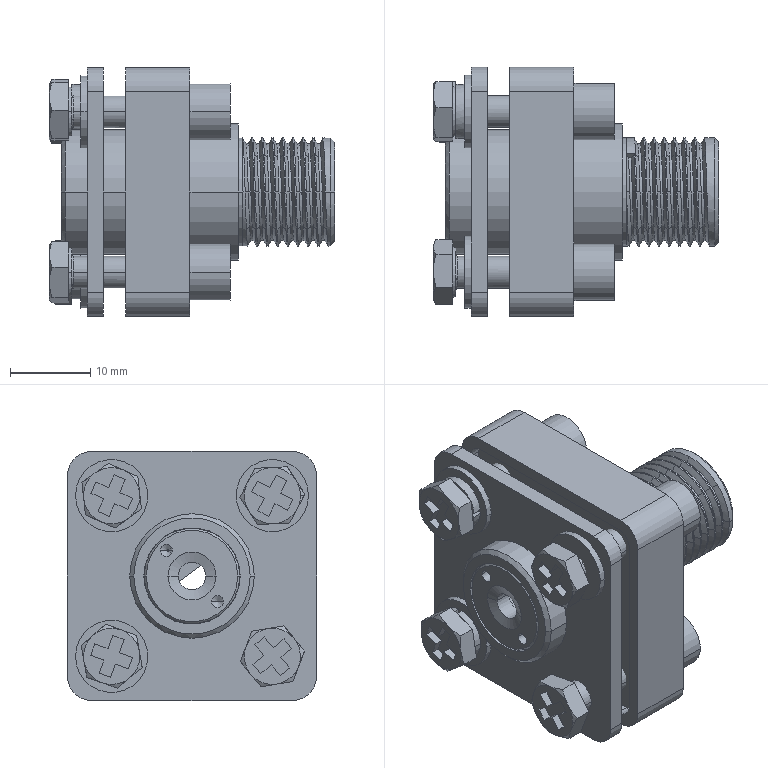Part | NX | features BREP 13 | 13 solids | 557 faces | box 35.5 x 31 x 31 mm | volume 13225 mm3 | spline 214 | plane 140 | cylinder 128 | cone 75 | commonest cylinder face diameters 13.458 x20 12.083 x16 4 x12 3.78 x10 7 x10 10 x10